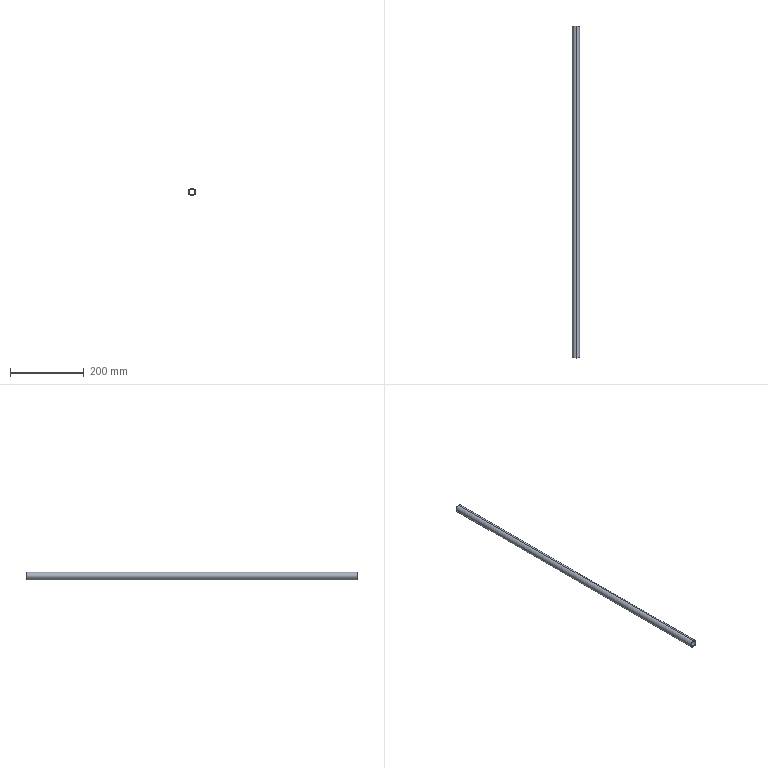Part | SolidWorks | features Sweep 1 | 1 solid | 6 faces | box 20 x 900 x 20 mm | volume 101788 mm3 | cylinder 4 | plane 2 | commonest cylinder face diameters 16 x2 20 x2
STEP:
#1=CARTESIAN_POINT('',(0.,0.,-8.));
#2=VERTEX_POINT('',#1);
#3=CARTESIAN_POINT('',(0.,0.,8.));
#4=VERTEX_POINT('',#3);
#5=CARTESIAN_POINT('',(0.,0.,0.));
#6=DIRECTION('',(0.,1.,0.));
#7=DIRECTION('',(0.,0.,1.));
#8=AXIS2_PLACEMENT_3D('',#5,#6,#7);
#9=CIRCLE('',#8,8.);
#10=EDGE_CURVE('',#2,#4,#9,.T.);
#11=ORIENTED_EDGE('',*,*,#10,.F.);
#12=CARTESIAN_POINT('',(0.,900.,-8.));
#13=VERTEX_POINT('',#12);
#14=CARTESIAN_POINT('',(0.,0.,-8.));
#15=DIRECTION('',(0.,1.,0.));
#16=VECTOR('',#15,1000.);
#17=LINE('',#14,#16);
#18=EDGE_CURVE('',#2,#13,#17,.T.);
#19=ORIENTED_EDGE('',*,*,#18,.T.);
#20=CARTESIAN_POINT('',(0.,900.,8.));
#21=VERTEX_POINT('',#20);
#22=CARTESIAN_POINT('',(0.,900.,0.));
#23=DIRECTION('',(0.,1.,0.));
#24=DIRECTION('',(0.,0.,1.));
#25=AXIS2_PLACEMENT_3D('',#22,#23,#24);
#26=CIRCLE('',#25,8.);
#27=EDGE_CURVE('',#13,#21,#26,.T.);
#28=ORIENTED_EDGE('',*,*,#27,.T.);
#29=CARTESIAN_POINT('',(0.,0.,8.));
#30=DIRECTION('',(0.,1.,0.));
#31=VECTOR('',#30,1000.);
#32=LINE('',#29,#31);
#33=EDGE_CURVE('',#4,#21,#32,.T.);
#34=ORIENTED_EDGE('',*,*,#33,.F.);
#35=EDGE_LOOP('',(#11,#19,#28,#34));
#36=FACE_OUTER_BOUND('',#35,.T.);
#37=CARTESIAN_POINT('',(0.,0.,0.));
#38=DIRECTION('',(0.,1.,0.));
#39=DIRECTION('',(0.,0.,1.));
#40=AXIS2_PLACEMENT_3D('',#37,#38,#39);
#41=CYLINDRICAL_SURFACE('',#40,8.);
#42=ADVANCED_FACE('',(#36),#41,.F.);
#43=CARTESIAN_POINT('',(0.,0.,10.));
#44=VERTEX_POINT('',#43);
#45=CARTESIAN_POINT('',(0.,0.,-10.));
#46=VERTEX_POINT('',#45);
#47=CARTESIAN_POINT('',(0.,0.,0.));
#48=DIRECTION('',(0.,1.,0.));
#49=DIRECTION('',(0.,0.,1.));
#50=AXIS2_PLACEMENT_3D('',#47,#48,#49);
#51=CIRCLE('',#50,10.);
#52=EDGE_CURVE('',#44,#46,#51,.T.);
#53=ORIENTED_EDGE('',*,*,#52,.T.);
#54=CARTESIAN_POINT('',(0.,900.,-10.));
#55=VERTEX_POINT('',#54);
#56=CARTESIAN_POINT('',(0.,0.,-10.));
#57=DIRECTION('',(0.,1.,0.));
#58=VECTOR('',#57,1000.);
#59=LINE('',#56,#58);
#60=EDGE_CURVE('',#46,#55,#59,.T.);
#61=ORIENTED_EDGE('',*,*,#60,.T.);
#62=CARTESIAN_POINT('',(0.,900.,10.));
#63=VERTEX_POINT('',#62);
#64=CARTESIAN_POINT('',(0.,900.,0.));
#65=DIRECTION('',(0.,1.,0.));
#66=DIRECTION('',(0.,0.,1.));
#67=AXIS2_PLACEMENT_3D('',#64,#65,#66);
#68=CIRCLE('',#67,10.);
#69=EDGE_CURVE('',#63,#55,#68,.T.);
#70=ORIENTED_EDGE('',*,*,#69,.F.);
#71=CARTESIAN_POINT('',(0.,0.,10.));
#72=DIRECTION('',(0.,1.,0.));
#73=VECTOR('',#72,1000.);
#74=LINE('',#71,#73);
#75=EDGE_CURVE('',#44,#63,#74,.T.);
#76=ORIENTED_EDGE('',*,*,#75,.F.);
#77=EDGE_LOOP('',(#53,#61,#70,#76));
#78=FACE_OUTER_BOUND('',#77,.T.);
#79=CARTESIAN_POINT('',(0.,0.,0.));
#80=DIRECTION('',(0.,1.,0.));
#81=DIRECTION('',(0.,0.,1.));
#82=AXIS2_PLACEMENT_3D('',#79,#80,#81);
#83=CYLINDRICAL_SURFACE('',#82,10.);
#84=ADVANCED_FACE('',(#78),#83,.T.);
#85=ORIENTED_EDGE('',*,*,#60,.F.);
#86=CARTESIAN_POINT('',(0.,0.,0.));
#87=DIRECTION('',(0.,1.,0.));
#88=DIRECTION('',(0.,0.,1.));
#89=AXIS2_PLACEMENT_3D('',#86,#87,#88);
#90=CIRCLE('',#89,10.);
#91=EDGE_CURVE('',#46,#44,#90,.T.);
#92=ORIENTED_EDGE('',*,*,#91,.T.);
#93=ORIENTED_EDGE('',*,*,#75,.T.);
#94=CARTESIAN_POINT('',(0.,900.,0.));
#95=DIRECTION('',(0.,1.,0.));
#96=DIRECTION('',(0.,0.,1.));
#97=AXIS2_PLACEMENT_3D('',#94,#95,#96);
#98=CIRCLE('',#97,10.);
#99=EDGE_CURVE('',#55,#63,#98,.T.);
#100=ORIENTED_EDGE('',*,*,#99,.F.);
#101=EDGE_LOOP('',(#85,#92,#93,#100));
#102=FACE_OUTER_BOUND('',#101,.T.);
#103=CARTESIAN_POINT('',(0.,0.,0.));
#104=DIRECTION('',(0.,1.,0.));
#105=DIRECTION('',(0.,0.,1.));
#106=AXIS2_PLACEMENT_3D('',#103,#104,#105);
#107=CYLINDRICAL_SURFACE('',#106,10.);
#108=ADVANCED_FACE('',(#102),#107,.T.);
#109=CARTESIAN_POINT('',(0.,900.,0.));
#110=DIRECTION('',(0.,1.,0.));
#111=DIRECTION('',(0.,0.,1.));
#112=AXIS2_PLACEMENT_3D('',#109,#110,#111);
#113=CIRCLE('',#112,8.);
#114=EDGE_CURVE('',#21,#13,#113,.T.);
#115=ORIENTED_EDGE('',*,*,#114,.F.);
#116=ORIENTED_EDGE('',*,*,#27,.F.);
#117=EDGE_LOOP('',(#115,#116));
#118=FACE_BOUND('',#117,.T.);
#119=ORIENTED_EDGE('',*,*,#69,.T.);
#120=ORIENTED_EDGE('',*,*,#99,.T.);
#121=EDGE_LOOP('',(#119,#120));
#122=FACE_OUTER_BOUND('',#121,.T.);
#123=CARTESIAN_POINT('',(0.,900.,0.));
#124=DIRECTION('',(0.,1.,0.));
#125=DIRECTION('',(0.,0.,1.));
#126=AXIS2_PLACEMENT_3D('',#123,#124,#125);
#127=PLANE('',#126);
#128=ADVANCED_FACE('',(#118,#122),#127,.T.);
#129=CARTESIAN_POINT('',(0.,0.,0.));
#130=DIRECTION('',(0.,1.,0.));
#131=DIRECTION('',(0.,0.,1.));
#132=AXIS2_PLACEMENT_3D('',#129,#130,#131);
#133=CIRCLE('',#132,8.);
#134=EDGE_CURVE('',#4,#2,#133,.T.);
#135=ORIENTED_EDGE('',*,*,#134,.T.);
#136=ORIENTED_EDGE('',*,*,#10,.T.);
#137=EDGE_LOOP('',(#135,#136));
#138=FACE_BOUND('',#137,.T.);
#139=ORIENTED_EDGE('',*,*,#52,.F.);
#140=ORIENTED_EDGE('',*,*,#91,.F.);
#141=EDGE_LOOP('',(#139,#140));
#142=FACE_OUTER_BOUND('',#141,.T.);
#143=CARTESIAN_POINT('',(0.,0.,0.));
#144=DIRECTION('',(0.,1.,0.));
#145=DIRECTION('',(0.,0.,1.));
#146=AXIS2_PLACEMENT_3D('',#143,#144,#145);
#147=PLANE('',#146);
#148=ADVANCED_FACE('',(#138,#142),#147,.F.);
#149=ORIENTED_EDGE('',*,*,#18,.F.);
#150=ORIENTED_EDGE('',*,*,#134,.F.);
#151=ORIENTED_EDGE('',*,*,#33,.T.);
#152=ORIENTED_EDGE('',*,*,#114,.T.);
#153=EDGE_LOOP('',(#149,#150,#151,#152));
#154=FACE_OUTER_BOUND('',#153,.T.);
#155=CARTESIAN_POINT('',(0.,0.,0.));
#156=DIRECTION('',(0.,1.,0.));
#157=DIRECTION('',(0.,0.,1.));
#158=AXIS2_PLACEMENT_3D('',#155,#156,#157);
#159=CYLINDRICAL_SURFACE('',#158,8.);
#160=ADVANCED_FACE('',(#154),#159,.F.);
#161=CLOSED_SHELL('',(#42,#84,#108,#128,#148,#160));
#162=MANIFOLD_SOLID_BREP('',#161);
#163=CARTESIAN_POINT('',(0.,0.,0.));
#164=DIRECTION('',(0.,0.,1.));
#165=DIRECTION('',(1.,0.,0.));
#166=AXIS2_PLACEMENT_3D('',#163,#164,#165);
#167=(LENGTH_UNIT()NAMED_UNIT(*)SI_UNIT(.MILLI.,.METRE.));
#168=UNCERTAINTY_MEASURE_WITH_UNIT(LENGTH_MEASURE(0.00001),#167,'','');
#169=(NAMED_UNIT(*)PLANE_ANGLE_UNIT()SI_UNIT($,.RADIAN.));
#170=(NAMED_UNIT(*)SI_UNIT($,.STERADIAN.)SOLID_ANGLE_UNIT());
#171=(GEOMETRIC_REPRESENTATION_CONTEXT(3)GLOBAL_UNCERTAINTY_ASSIGNED_CONTEXT((#168))GLOBAL_UNIT_ASSIGNED_CONTEXT((#167,#169,#170))REPRESENTATION_CONTEXT('',''));
#172=ADVANCED_BREP_SHAPE_REPRESENTATION('',(#162,#166),#171);